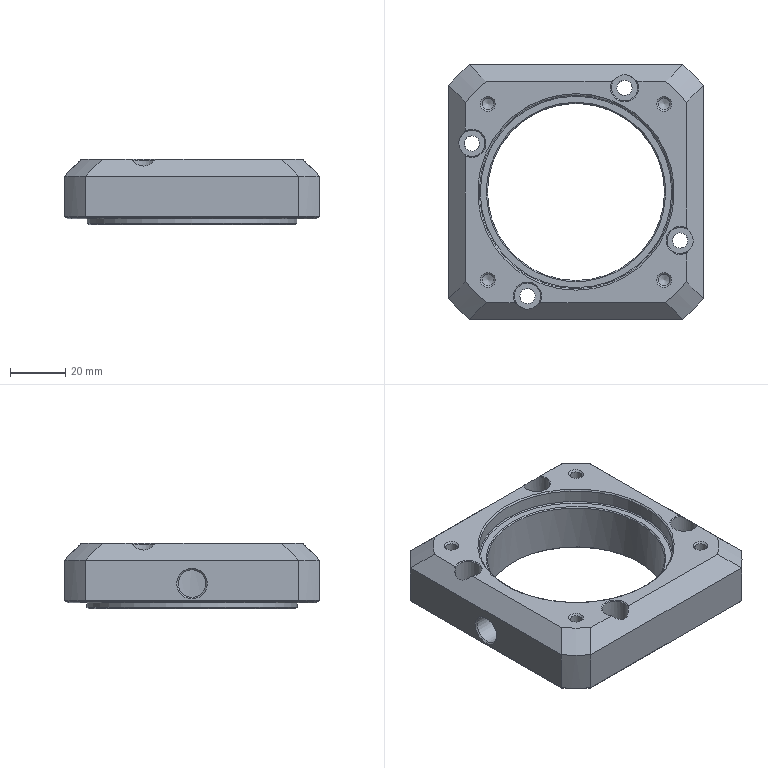Part | STEP file | SOLID | 1 solid | 70 faces | box 92 x 92 x 23.5 mm | volume 95291 mm3 | cone 22 | plane 21 | cylinder 20 | spline 4 | torus 3 | commonest cylinder face diameters 4.2 x4 5.5 x4 9.5 x4 120 x4 10 x1 64 x1